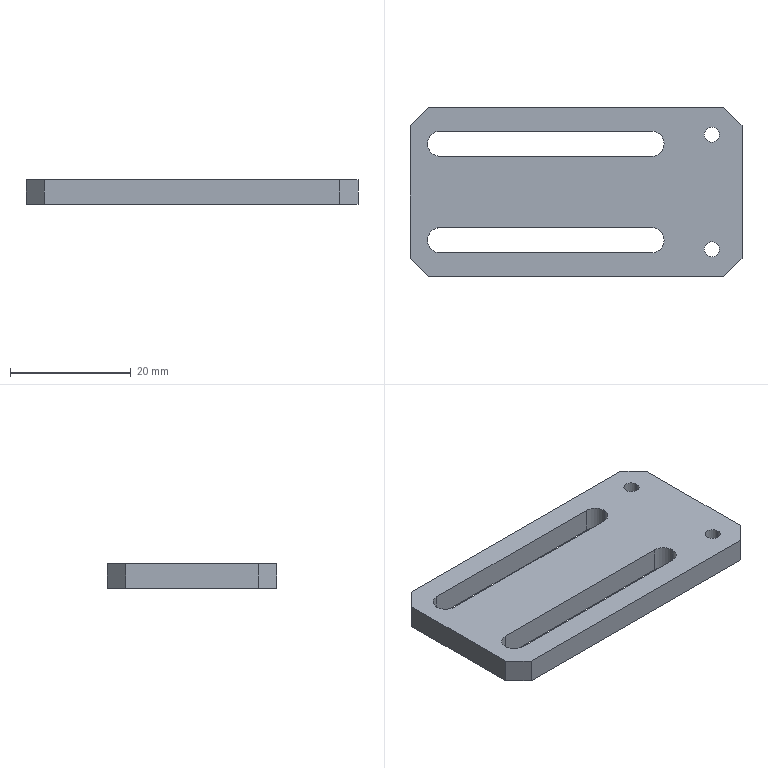Part | STEP file | 0-22 Sensor seat | 1 solid | 24 faces | box 55 x 28 x 4 mm | volume 4762 mm3 | plane 14 | cylinder 10 | commonest cylinder face diameters 4.2 x6 2.5 x4